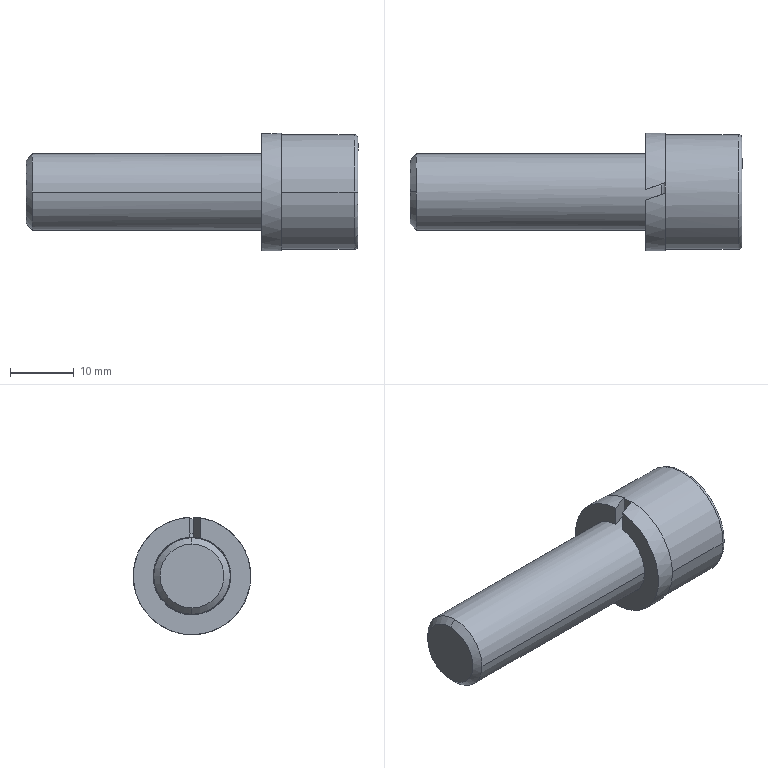Part | STEP file | Positioning_id1598_x_t | 1 solid | 26 faces | box 52 x 18.4 x 18.398 mm | volume 7494 mm3 | plane 14 | cylinder 6 | torus 4 | cone 2 | commonest cylinder face diameters 12 x2 18 x2 12.2 x1 18.4 x1